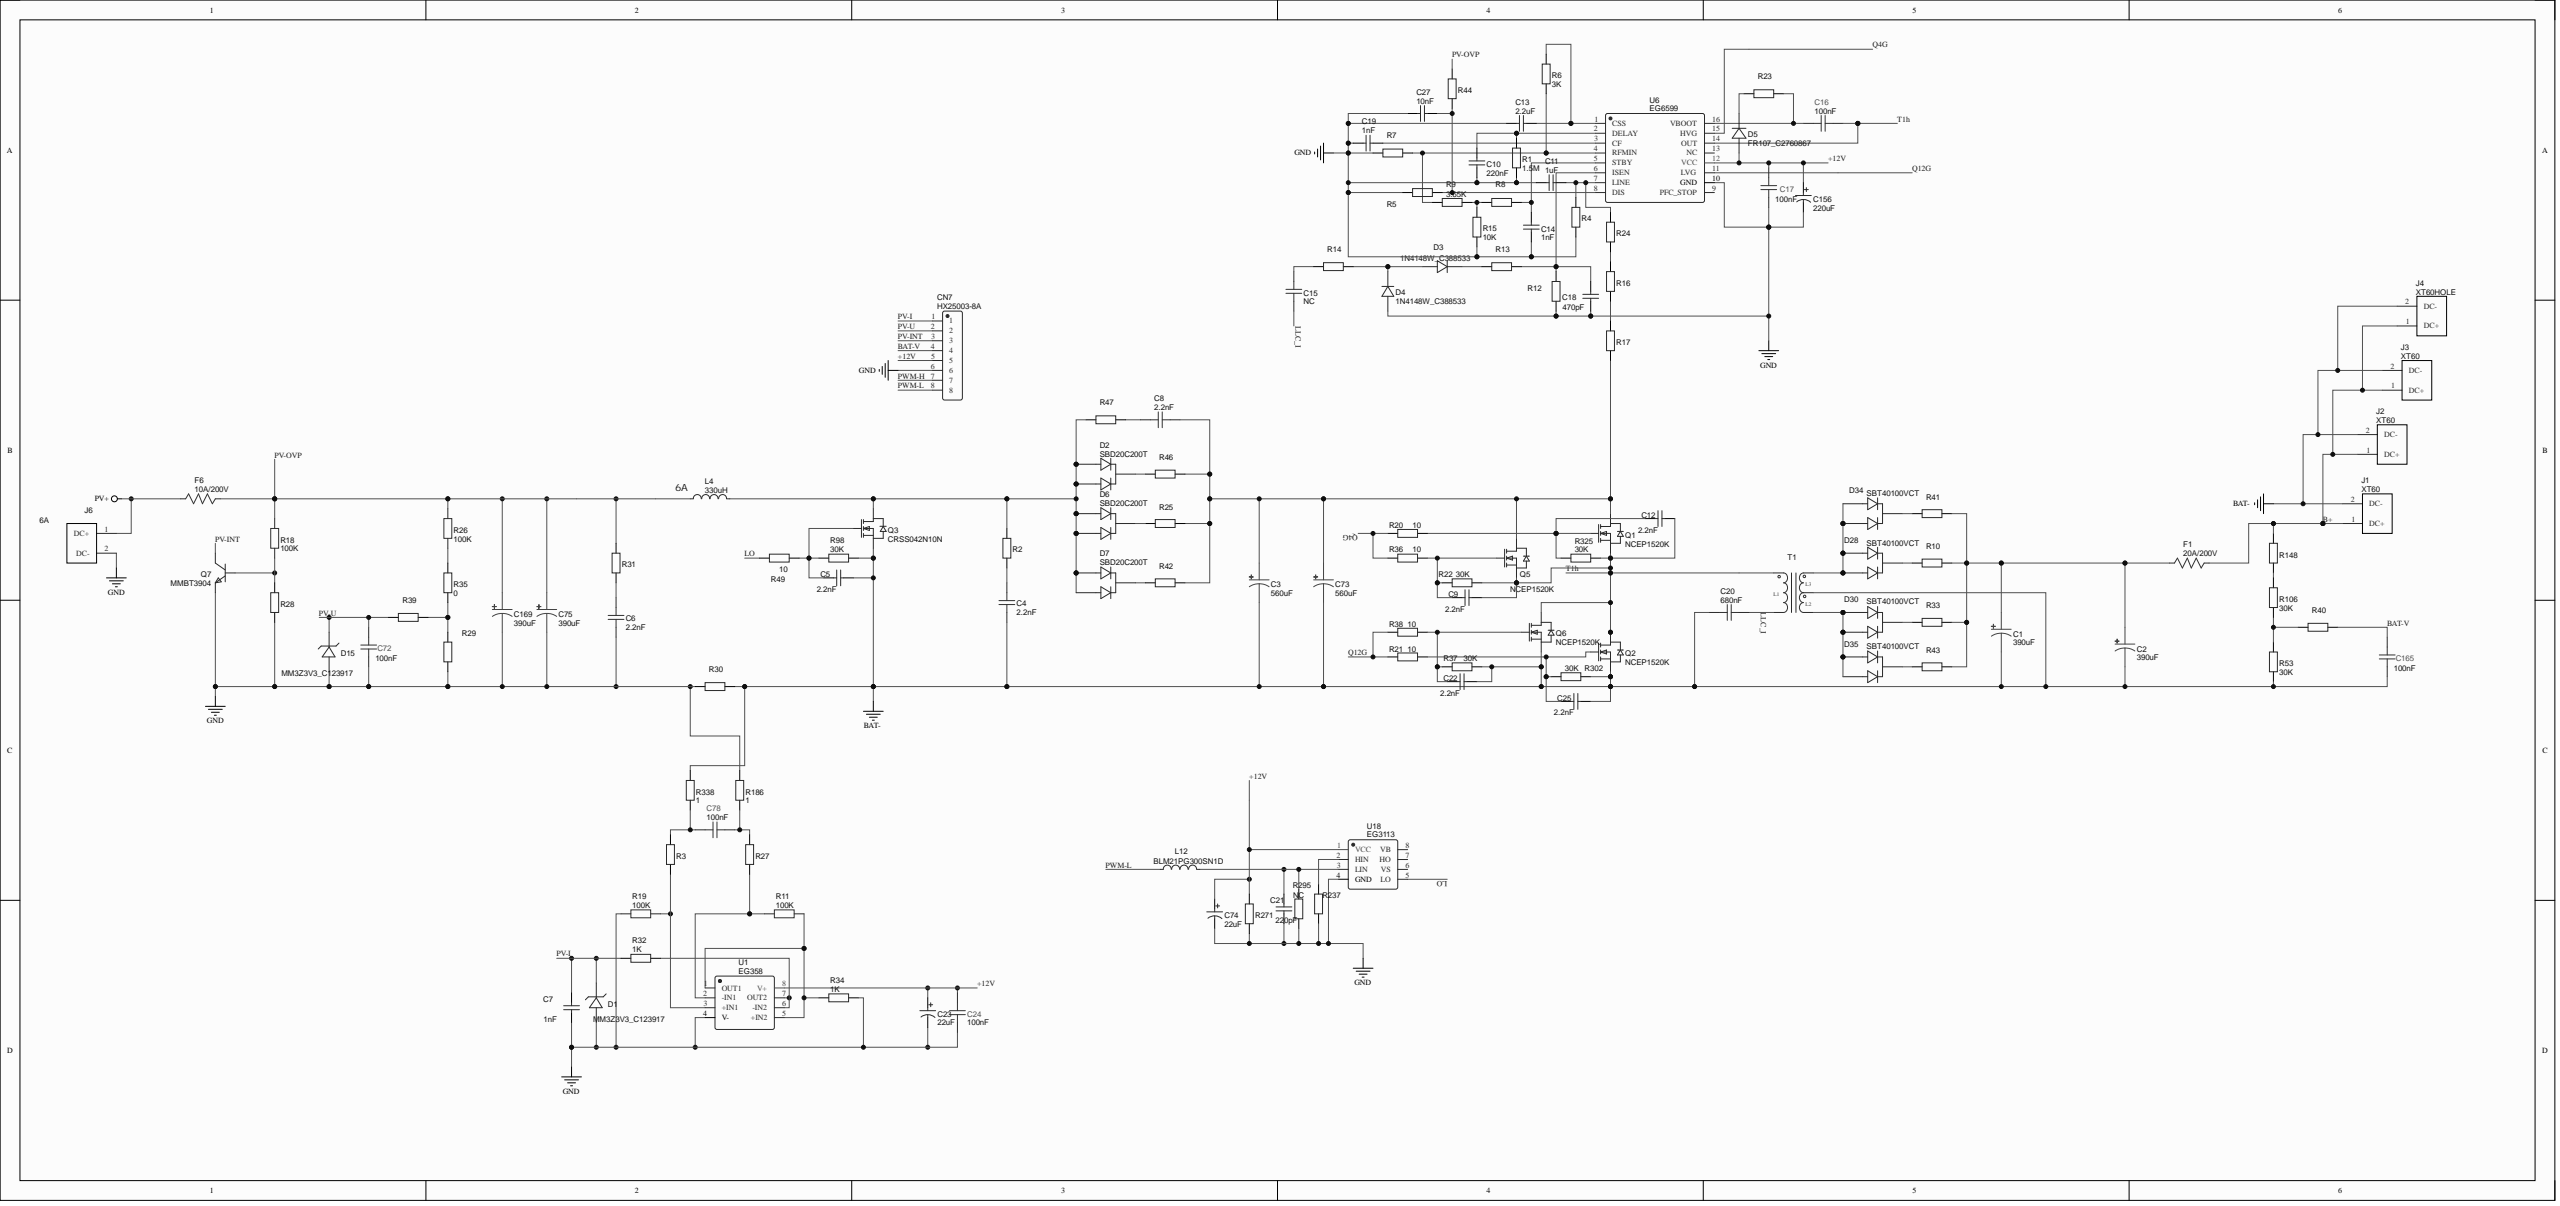Circuit board | Altium Designer | 124 parts | 65 nets
Bill of materials:
Comment,Description,Designator,Footprint,LibRef,Quantity
"390uF","","C1, C2","CAP-TH_BD8.0-P3.50-D0.6-FD","390uF","2"
"560uF","","C3, C73","CAP-TH_BD12.5-P5.00-D0.6-FD","560uF","2"
"2.2nF","","C4, C6, C8","C1206","2.2nF","3"
"2.2nF","","C5, C9, C12, C22, C25","C0603","2.2nF","5"
"1nF","","C7, C14, C19","C0603","1nF","3"
"220nF","","C10","C0603","220nF","1"
"1uF","","C11","C0603","1uF","1"
"2.2uF","","C13","C0603","2.2uF","1"
"NC","","C15","C1206","NC","1"
"100nF","","C16, C17, C24, C72, C78, C165","C0603","100nF","6"
"470pF","","C18","C0603","470pF","1"
"680nF","","C20","CAP-TH_L17.5-W8.5-P15.00-D0.8","680nF","1"
"220pF","","C21","C0603","220pF","1"
"22uF","","C23, C74","CAP-TH_BD5.0-P2.00-D0.8-FD","22uF","2"
"10nF","","C27","C1206","10nF","1"
"390uF","","C75, C169","CAP-TH_BD10.0-P5.00-D1.0-FD","390uF","2"
"220uF","","C156","CAP-TH_BD6.3-P2.50-D1.0-FD","220uF","1"
"HX25003-8A","","CN7","CONN-TH_8P-P2.50_HX25003-8A","HX25003-8A","1"
"MM3Z3V3_C123917","","D1, D15","SOD-323_L1.8-W1.3-LS2.5-RD","MM3Z3V3_C123917","2"
"SBD20C200T","","D2, D6, D7","TO-220-3_L10.0-W4.5-P2.54-L","SBD20C200T","3"
"1N4148W_C388533","","D3, D4","SOD-123_L2.8-W1.8-LS3.7-RD","1N4148W_C388533","2"
"FR107_C2760867","","D5","SOD-123FL_L2.7-W1.8-LS3.8-RD","FR107_C2760867","1"
"SBT40100VCT","","D28, D30, D34, D35","TO-220-3_L10.0-W4.5-P2.54-L","SBT40100VCT","4"
"20A/200V","","F1","FUSE-SMD_L6.1-W2.5","20A/200V","1"
"10A/200V","","F6","FUSE-SMD_L6.1-W2.5","10A/200V","1"
"XT60","","J1, J2, J3","CONN-TH_XT60UPB-F","XT60","3"
"XT60HOLE","","J4","XT90N","XT60HOLE","1"
"6A","","J6","CONN-TH_XT60UPB-F","6A","1"
"330uH","","L4","200W-TMS330060A","330uH","1"
"BLM21PG300SN1D","","L12","L0805","BLM21PG300SN1D","1"
"NCEP1520K","","Q1, Q2, Q5, Q6","TO-252-2_L6.6-W6.1-P4.57-LS9.9-BR-CW","NCEP1520K","4"
"CRSS042N10N","","Q3","TO-263-3_L10.2-W10.7-P5.08-LS16.2-TL","CRSS042N10N","1"
"MMBT3904","","Q7","SOT-23-3_L2.9-W1.3-P1.90-LS2.4-BR","MMBT3904","1"
"1.5M","","R1","R0603","1.5M","1"
"","","R2, R17, R31, R47","R1206","","4"
"","","R3, R4, R7, R8, R12, R13, R14, R16, R24, R27, R29, R148, R237, R271","R0603","","14"
"","","R5, R23, R28, R39, R40, R44","R0805","","6"
"3K","","R6","R0603","3K","1"
"3.65K","","R9","R0603","3.65K","1"
"","","R10, R25, R30, R33, R41, R42, R43, R46","R2512","","8"
"100K","","R11, R18, R19, R26","R0805","100K","4"
"10K","","R15","R1206","10K","1"
"10","","R20, R21, R36, R38","R1206","10","4"
"30K","","R22, R37, R53, R98, R106, R302, R325","R0603","30K","7"
"1K","","R32, R34","R0603","1K","2"
"0","","R35","R0805","0","1"
"10","","R49","R0603","10","1"
"1","","R186, R338","R0603","1","2"
"NC","","R295","R0603","NC","1"
"","","T1","PQ3230 3:2:2-N","","1"
"EG358","","U1","SOIC-8_L5.0-W4.0-P1.27-LS6.0-BL","EG358","1"
"EG6599","","U6","SO-16_L10.0-W4.0-P1.27-LS6.2-BL","EG6599","1"
"EG3113","","U18","SOP-8_L4.9-W3.9-P1.27-LS6.0-BL","EG3113","1"
Netlist (Protel format):
[
C1
CAP-TH_BD8.0-P3.50-D0.6-FD
390uF



]
[
C2
CAP-TH_BD8.0-P3.50-D0.6-FD
390uF



]
[
C3
CAP-TH_BD12.5-P5.00-D0.6-FD
560uF



]
[
C4
C1206
2.2nF



]
[
C5
C0603
2.2nF



]
[
C6
C1206
2.2nF



]
[
C7
C0603
1nF



]
[
C8
C1206
2.2nF



]
[
C9
C0603
2.2nF



]
[
C10
C0603
220nF



]
[
C11
C0603
1uF



]
[
C12
C0603
2.2nF



]
[
C13
C0603
2.2uF



]
[
C14
C0603
1nF



]
[
C15
C1206
NC



]
[
C16
C0603
100nF



]
[
C17
C0603
100nF



]
[
C18
C0603
470pF



]
[
C19
C0603
1nF



]
[
C20
CAP-TH_L17.5-W8.5-P15.00-D0.8
680nF



]
[
C21
C0603
220pF



]
[
C22
C0603
2.2nF



]
[
C23
CAP-TH_BD5.0-P2.00-D0.8-FD
22uF



]
[
C24
C0603
100nF



]
[
C25
C0603
2.2nF



]
[
C27
C1206
10nF



]
[
C72
C0603
100nF



]
[
C73
CAP-TH_BD12.5-P5.00-D0.6-FD
560uF



]
[
C74
CAP-TH_BD5.0-P2.00-D0.8-FD
22uF



]
[
C75
CAP-TH_BD10.0-P5.00-D1.0-FD
390uF



]
[
C78
C0603
100nF



]
[
C156
CAP-TH_BD6.3-P2.50-D1.0-FD
220uF



]
[
C165
C0603
100nF



]
[
C169
CAP-TH_BD10.0-P5.00-D1.0-FD
390uF



]
[
CN7
CONN-TH_8P-P2.50_HX25003-8A
HX25003-8A



]
[
D1
SOD-323_L1.8-W1.3-LS2.5-RD
MM3Z3V3_C123917



]
[
D2
TO-220-3_L10.0-W4.5-P2.54-L
SBD20C200T



]
[
D3
SOD-123_L2.8-W1.8-LS3.7-RD
1N4148W_C388533



]
[
D4
SOD-123_L2.8-W1.8-LS3.7-RD
1N4148W_C388533



]
[
D5
SOD-123FL_L2.7-W1.8-LS3.8-RD
FR107_C2760867



]
[
D6
TO-220-3_L10.0-W4.5-P2.54-L
SBD20C200T



]
[
D7
TO-220-3_L10.0-W4.5-P2.54-L
SBD20C200T



]
[
D15
SOD-323_L1.8-W1.3-LS2.5-RD
MM3Z3V3_C123917



]
[
D28
TO-220-3_L10.0-W4.5-P2.54-L
SBT40100VCT



]
[
D30
TO-220-3_L10.0-W4.5-P2.54-L
SBT40100VCT



]
[
D34
TO-220-3_L10.0-W4.5-P2.54-L
SBT40100VCT



]
[
D35
TO-220-3_L10.0-W4.5-P2.54-L
SBT40100VCT



]
[
F1
FUSE-SMD_L6.1-W2.5
20A/200V



]
[
F6
FUSE-SMD_L6.1-W2.5
10A/200V



]
[
J1
CONN-TH_XT60UPB-F
XT60



]
[
J2
CONN-TH_XT60UPB-F
XT60



]
[
J3
CONN-TH_XT60UPB-F
XT60



]
[
J4
XT90N
XT60HOLE



]
[
J6
CONN-TH_XT60UPB-F
6A



]
[
L4
200W-TMS330060A
330uH



]
[
L12
L0805
BLM21PG300SN1D



]
[
Q1
TO-252-2_L6.6-W6.1-P4.57-LS9.9-BR-CW
NCEP1520K



]
[
Q2
TO-252-2_L6.6-W6.1-P4.57-LS9.9-BR-CW
NCEP1520K



]
[
Q3
TO-263-3_L10.2-W10.7-P5.08-LS16.2-TL
CRSS042N10N



]
[
Q5
TO-252-2_L6.6-W6.1-P4.57-LS9.9-BR-CW
NCEP1520K



]
[
Q6
TO-252-2_L6.6-W6.1-P4.57-LS9.9-BR-CW
NCEP1520K



]
[
Q7
SOT-23-3_L2.9-W1.3-P1.90-LS2.4-BR
MMBT3904



]
[
R1
R0603
1.5M



]
[
R2
R1206




]
[
R3
R0603




]
[
R4
R0603




]
[
R5
R0805




]
[
R6
R0603
3K



]
[
R7
R0603




]
[
R8
R0603




]
[
R9
R0603
3.65K



]
[
R10
R2512




]
[
R11
R0805
100K



]
[
R12
R0603




]
[
R13
R0603




]
[
R14
R0603




]
[
R15
R1206
10K



]
[
R16
R0603




]
[
R17
R1206




]
[
R18
R0805
100K



]
[
R19
R0805
100K



]
[
R20
R1206
10



]
[
R21
R1206
10



]
[
R22
R0603
30K



]
[
R23
R0805




]
[
R24
R0603




]
[
R25
R2512




]
[
R26
R0805
100K



]
[
R27
R0603




]
[
R28
R0805




]
[
R29
R0603




]
[
R30
R2512




]
[
R31
R1206




]
[
R32
R0603
1K



]
[
R33
R2512




]
[
R34
R0603
1K



]
[
R35
R0805
0



]
[
R36
R1206
10



]
[
R37
R0603
30K



]
[
R38
R1206
10



]
[
R39
R0805




]
[
R40
R0805




]
[
R41
R2512




]
[
R42
R2512




]
[
R43
R2512




]
[
R44
R0805




]
[
R46
R2512




]
[
R47
R1206




]
[
R49
R0603
10



]
[
R53
R0603
30K



]
[
R98
R0603
30K



]
[
R106
R0603
30K



]
[
R148
R0603




]
[
R186
R0603
1



]
[
R237
R0603




]
[
R271
R0603




]
[
R295
R0603
NC



]
[
R302
R0603
30K



]
[
R325
R0603
30K



]
[
R338
R0603
1



]
[
T1
PQ3230 3:2:2-N




]
[
U1
SOIC-8_L5.0-W4.0-P1.27-LS6.0-BL
EG358



]
[
U6
SO-16_L10.0-W4.0-P1.27-LS6.2-BL
EG6599



]
[
U18
SOP-8_L4.9-W3.9-P1.27-LS6.0-BL
EG3113



]
(
T1h
C9-2
C12-2
C16-1
Q1-3
Q2-2
Q5-3
Q6-2
R22-2
R325-2
T1-4
U6-14
)
(
Q12G
R21-1
R38-1
U6-11
)
(
Q4G
R20-1
R36-1
U6-15
)
(
PWM-L
CN7-8
L12-1
)
(
PV-U
C72-2
CN7-2
D15-1
R39-1
)
(
PV-OVP
C75-1
C169-1
F6-2
L4-1
R18-2
R26-2
R31-1
R44-2
)
(
PV-INT
CN7-3
Q7-3
)
(
PV-I
C7-2
CN7-1
D1-1
R32-2
)
(
PV+
F6-1
J6-1
)
(
NetR237_2
R237-2
U18-2
)
(
NetR106_2
R106-2
R148-1
)
(
NetR40_1
R40-1
R53-2
R106-1
)
(
NetR32_1
R32-1
U1-6
U1-7
)
(
NetR29_2
R29-2
R35-1
R39-2
)
(
NetR26_1
R26-1
R35-2
)
(
NetR16_2
R16-2
R24-1
)
(
NetR16_1
R16-1
R17-2
)
(
NetR11_2
R11-2
R27-1
U1-2
)
(
NetR11_1
R11-1
R34-1
U1-1
U1-5
)
(
NetR8_1
R8-1
R9-2
R15-1
)
(
NetR6_1
R6-1
R7-1
R9-1
U6-4
)
(
NetR3_1
R3-1
R19-1
U1-3
)
(
NetQ7_1
Q7-1
R18-1
R28-2
)
(
NetD35_2
D35-2
R43-1
)
(
NetD34_2
D34-2
R41-1
)
(
NetD30_2
D30-2
R33-1
)
(
NetD30_1
D30-1
D30-3
D35-1
D35-3
T1-10
)
(
NetD28_2
D28-2
R10-1
)
(
NetD28_1
D28-1
D28-3
D34-1
D34-3
T1-8
)
(
NetD7_2
D7-2
R42-1
)
(
NetD6_2
D6-2
R25-1
)
(
NetD5_1
D5-1
R23-2
)
(
NetD3_2
D3-2
D4-1
R14-2
)
(
NetD3_1
D3-1
R13-1
)
(
NetD2_2
D2-2
R46-1
)
(
NetD2_1
D2-1
D2-3
D6-1
D6-3
D7-1
D7-3
L4-2
Q3-2
R2-1
R47-1
)
(
NetC78_2
C78-2
R3-2
R338-1
)
(
NetC78_1
C78-1
R27-2
R186-1
)
(
NetC27_2
C27-2
R5-2
R44-1
U6-8
)
(
NetC25_1
C25-1
Q2-1
R21-2
R302-1
)
(
NetC22_1
C22-1
Q6-1
R37-1
R38-2
)
(
NetC21_2
C21-2
L12-2
R295-1
U18-3
)
(
NetC19_1
C19-1
U6-3
)
(
NetC18_2
C18-2
R12-2
R13-2
U6-6
)
(
NetC16_2
C16-2
R23-1
U6-16
)
(
NetC15_2
C15-2
R14-1
)
(
NetC14_2
C14-2
R8-2
U6-5
)
(
NetC13_2
C13-2
R6-2
U6-1
)
(
NetC12_1
C12-1
Q1-1
R20-2
R325-1
)
(
NetC11_1
C11-1
R4-2
R24-2
U6-7
)
(
NetC10_2
C10-2
R1-2
U6-2
)
(
NetC9_1
C9-1
Q5-1
R22-1
R36-2
)
(
NetC8_1
C8-1
R47-2
)
(
NetC6_1
C6-1
R31-2
)
(
NetC5_1
C5-1
Q3-1
R49-1
R98-2
)
(
NetC4_1
C4-1
R2-2
)
(
NetC3_1
C3-1
C8-2
C73-1
Q1-2
Q5-2
R17-1
R25-2
R42-2
R46-2
)
(
NetC1_1
C1-1
C2-1
F1-1
R10-2
R33-2
R41-2
R43-2
)
(
LO
R49-2
U18-5
)
(
LLC_I
C15-1
C20-1
T1-3
)
(
GND
C6-2
C7-1
C10-1
C11-2
C13-1
C14-1
C17-1
C18-1
C19-2
C21-1
C23-2
C24-2
C27-1
C72-1
C74-2
C75-2
C156-2
C169-2
CN7-6
D1-2
D4-2
D15-2
J6-2
Q7-2
R1-1
R4-1
R5-1
R7-2
R12-1
R15-2
R19-2
R28-1
R29-1
R30-1
R34-2
R186-2
R237-1
R271-1
R295-2
U1-4
U6-10
U18-4
)
(
BAT-V
C165-2
CN7-4
R40-2
)
(
BAT-
C1-2
C2-2
C3-2
C4-2
C5-2
C20-2
C22-2
C25-2
C73-2
C165-1
J1-2
J2-2
J3-2
J4-2
Q2-3
Q3-3
Q6-3
R30-2
R37-2
R53-1
R98-1
R302-2
R338-2
T1-9
)
(
B+
F1-2
J1-1
J2-1
J3-1
J4-1
R148-2
)
(
+12V
C17-2
C23-1
C24-1
C74-1
C156-1
CN7-5
D5-2
R271-2
U1-8
U6-12
U18-1
)